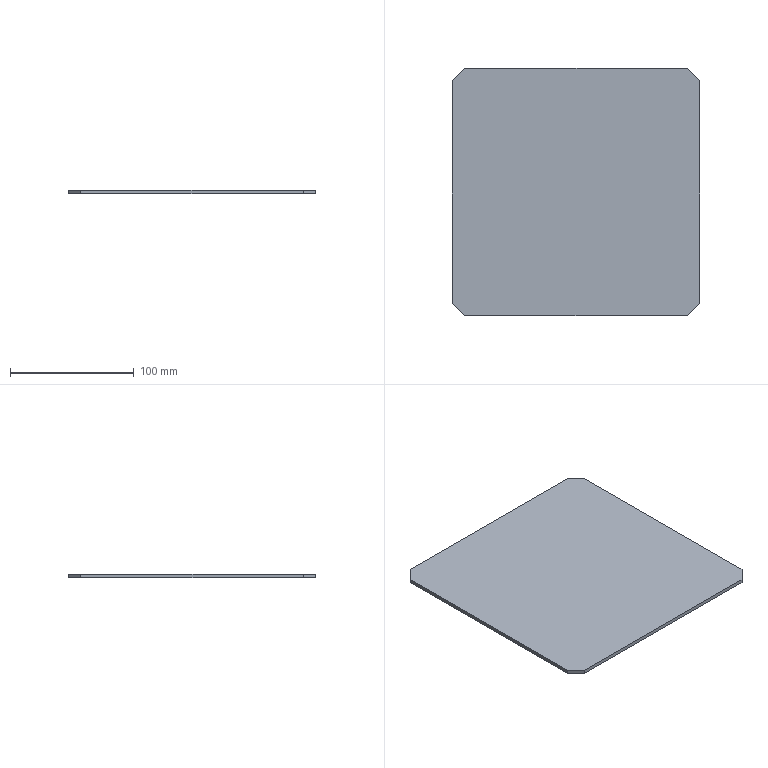Part | SolidWorks | features Chamfer 1, Extrusion 1 | 1 solid | 10 faces | box 200 x 200 x 3 mm | volume 119400 mm3 | plane 10
STEP:
#1=CARTESIAN_POINT('',(100.,-90.,3.));
#2=VERTEX_POINT('',#1);
#3=CARTESIAN_POINT('',(100.,90.,3.));
#4=VERTEX_POINT('',#3);
#5=CARTESIAN_POINT('',(100.,100.,3.));
#6=DIRECTION('',(0.,1.,0.));
#7=VECTOR('',#6,1000.);
#8=LINE('',#5,#7);
#9=EDGE_CURVE('',#2,#4,#8,.T.);
#10=ORIENTED_EDGE('',*,*,#9,.F.);
#11=CARTESIAN_POINT('',(100.,-90.,0.));
#12=VERTEX_POINT('',#11);
#13=CARTESIAN_POINT('',(100.,-90.,3.));
#14=DIRECTION('',(0.,0.,-1.));
#15=VECTOR('',#14,1000.);
#16=LINE('',#13,#15);
#17=EDGE_CURVE('',#2,#12,#16,.T.);
#18=ORIENTED_EDGE('',*,*,#17,.T.);
#19=CARTESIAN_POINT('',(100.,90.,0.));
#20=VERTEX_POINT('',#19);
#21=CARTESIAN_POINT('',(100.,100.,0.));
#22=DIRECTION('',(0.,1.,0.));
#23=VECTOR('',#22,1000.);
#24=LINE('',#21,#23);
#25=EDGE_CURVE('',#12,#20,#24,.T.);
#26=ORIENTED_EDGE('',*,*,#25,.T.);
#27=CARTESIAN_POINT('',(100.,90.,3.));
#28=DIRECTION('',(0.,0.,1.));
#29=VECTOR('',#28,1000.);
#30=LINE('',#27,#29);
#31=EDGE_CURVE('',#20,#4,#30,.T.);
#32=ORIENTED_EDGE('',*,*,#31,.T.);
#33=EDGE_LOOP('',(#10,#18,#26,#32));
#34=FACE_OUTER_BOUND('',#33,.T.);
#35=CARTESIAN_POINT('',(100.,100.,3.));
#36=DIRECTION('',(-1.,0.,0.));
#37=DIRECTION('',(0.,-1.,0.));
#38=AXIS2_PLACEMENT_3D('',#35,#36,#37);
#39=PLANE('',#38);
#40=ADVANCED_FACE('',(#34),#39,.F.);
#41=CARTESIAN_POINT('',(90.,100.,3.));
#42=VERTEX_POINT('',#41);
#43=CARTESIAN_POINT('',(-90.,100.,3.));
#44=VERTEX_POINT('',#43);
#45=CARTESIAN_POINT('',(-100.,100.,3.));
#46=DIRECTION('',(-1.,0.,0.));
#47=VECTOR('',#46,1000.);
#48=LINE('',#45,#47);
#49=EDGE_CURVE('',#42,#44,#48,.T.);
#50=ORIENTED_EDGE('',*,*,#49,.F.);
#51=CARTESIAN_POINT('',(90.,100.,0.));
#52=VERTEX_POINT('',#51);
#53=CARTESIAN_POINT('',(90.,100.,3.));
#54=DIRECTION('',(0.,0.,-1.));
#55=VECTOR('',#54,1000.);
#56=LINE('',#53,#55);
#57=EDGE_CURVE('',#42,#52,#56,.T.);
#58=ORIENTED_EDGE('',*,*,#57,.T.);
#59=CARTESIAN_POINT('',(-90.,100.,0.));
#60=VERTEX_POINT('',#59);
#61=CARTESIAN_POINT('',(-100.,100.,0.));
#62=DIRECTION('',(-1.,0.,0.));
#63=VECTOR('',#62,1000.);
#64=LINE('',#61,#63);
#65=EDGE_CURVE('',#52,#60,#64,.T.);
#66=ORIENTED_EDGE('',*,*,#65,.T.);
#67=CARTESIAN_POINT('',(-90.,100.,3.));
#68=DIRECTION('',(0.,0.,1.));
#69=VECTOR('',#68,1000.);
#70=LINE('',#67,#69);
#71=EDGE_CURVE('',#60,#44,#70,.T.);
#72=ORIENTED_EDGE('',*,*,#71,.T.);
#73=EDGE_LOOP('',(#50,#58,#66,#72));
#74=FACE_OUTER_BOUND('',#73,.T.);
#75=CARTESIAN_POINT('',(-100.,100.,3.));
#76=DIRECTION('',(0.,-1.,0.));
#77=DIRECTION('',(0.,0.,-1.));
#78=AXIS2_PLACEMENT_3D('',#75,#76,#77);
#79=PLANE('',#78);
#80=ADVANCED_FACE('',(#74),#79,.F.);
#81=CARTESIAN_POINT('',(-100.,90.,0.));
#82=VERTEX_POINT('',#81);
#83=CARTESIAN_POINT('',(-100.,-90.,0.));
#84=VERTEX_POINT('',#83);
#85=CARTESIAN_POINT('',(-100.,100.,0.));
#86=DIRECTION('',(0.,-1.,0.));
#87=VECTOR('',#86,1000.);
#88=LINE('',#85,#87);
#89=EDGE_CURVE('',#82,#84,#88,.T.);
#90=ORIENTED_EDGE('',*,*,#89,.T.);
#91=CARTESIAN_POINT('',(-100.,-90.,3.));
#92=VERTEX_POINT('',#91);
#93=CARTESIAN_POINT('',(-100.,-90.,3.));
#94=DIRECTION('',(0.,0.,1.));
#95=VECTOR('',#94,1000.);
#96=LINE('',#93,#95);
#97=EDGE_CURVE('',#84,#92,#96,.T.);
#98=ORIENTED_EDGE('',*,*,#97,.T.);
#99=CARTESIAN_POINT('',(-100.,90.,3.));
#100=VERTEX_POINT('',#99);
#101=CARTESIAN_POINT('',(-100.,100.,3.));
#102=DIRECTION('',(0.,-1.,0.));
#103=VECTOR('',#102,1000.);
#104=LINE('',#101,#103);
#105=EDGE_CURVE('',#100,#92,#104,.T.);
#106=ORIENTED_EDGE('',*,*,#105,.F.);
#107=CARTESIAN_POINT('',(-100.,90.,3.));
#108=DIRECTION('',(0.,0.,-1.));
#109=VECTOR('',#108,1000.);
#110=LINE('',#107,#109);
#111=EDGE_CURVE('',#100,#82,#110,.T.);
#112=ORIENTED_EDGE('',*,*,#111,.T.);
#113=EDGE_LOOP('',(#90,#98,#106,#112));
#114=FACE_OUTER_BOUND('',#113,.T.);
#115=CARTESIAN_POINT('',(-100.,100.,3.));
#116=DIRECTION('',(1.,0.,0.));
#117=DIRECTION('',(0.,1.,0.));
#118=AXIS2_PLACEMENT_3D('',#115,#116,#117);
#119=PLANE('',#118);
#120=ADVANCED_FACE('',(#114),#119,.F.);
#121=CARTESIAN_POINT('',(-90.,-100.,3.));
#122=VERTEX_POINT('',#121);
#123=CARTESIAN_POINT('',(90.,-100.,3.));
#124=VERTEX_POINT('',#123);
#125=CARTESIAN_POINT('',(-100.,-100.,3.));
#126=DIRECTION('',(1.,0.,0.));
#127=VECTOR('',#126,1000.);
#128=LINE('',#125,#127);
#129=EDGE_CURVE('',#122,#124,#128,.T.);
#130=ORIENTED_EDGE('',*,*,#129,.F.);
#131=CARTESIAN_POINT('',(-90.,-100.,0.));
#132=VERTEX_POINT('',#131);
#133=CARTESIAN_POINT('',(-90.,-100.,3.));
#134=DIRECTION('',(0.,0.,-1.));
#135=VECTOR('',#134,1000.);
#136=LINE('',#133,#135);
#137=EDGE_CURVE('',#122,#132,#136,.T.);
#138=ORIENTED_EDGE('',*,*,#137,.T.);
#139=CARTESIAN_POINT('',(90.,-100.,0.));
#140=VERTEX_POINT('',#139);
#141=CARTESIAN_POINT('',(-100.,-100.,0.));
#142=DIRECTION('',(1.,0.,0.));
#143=VECTOR('',#142,1000.);
#144=LINE('',#141,#143);
#145=EDGE_CURVE('',#132,#140,#144,.T.);
#146=ORIENTED_EDGE('',*,*,#145,.T.);
#147=CARTESIAN_POINT('',(90.,-100.,3.));
#148=DIRECTION('',(0.,0.,1.));
#149=VECTOR('',#148,1000.);
#150=LINE('',#147,#149);
#151=EDGE_CURVE('',#140,#124,#150,.T.);
#152=ORIENTED_EDGE('',*,*,#151,.T.);
#153=EDGE_LOOP('',(#130,#138,#146,#152));
#154=FACE_OUTER_BOUND('',#153,.T.);
#155=CARTESIAN_POINT('',(-100.,-100.,3.));
#156=DIRECTION('',(0.,1.,0.));
#157=DIRECTION('',(0.,0.,1.));
#158=AXIS2_PLACEMENT_3D('',#155,#156,#157);
#159=PLANE('',#158);
#160=ADVANCED_FACE('',(#154),#159,.F.);
#161=ORIENTED_EDGE('',*,*,#105,.T.);
#162=CARTESIAN_POINT('',(-95.,-95.,3.));
#163=DIRECTION('',(0.7071,-0.7071,0.));
#164=VECTOR('',#163,1000.);
#165=LINE('',#162,#164);
#166=EDGE_CURVE('',#92,#122,#165,.T.);
#167=ORIENTED_EDGE('',*,*,#166,.T.);
#168=ORIENTED_EDGE('',*,*,#129,.T.);
#169=CARTESIAN_POINT('',(95.,-95.,3.));
#170=DIRECTION('',(0.7071,0.7071,0.));
#171=VECTOR('',#170,1000.);
#172=LINE('',#169,#171);
#173=EDGE_CURVE('',#124,#2,#172,.T.);
#174=ORIENTED_EDGE('',*,*,#173,.T.);
#175=ORIENTED_EDGE('',*,*,#9,.T.);
#176=CARTESIAN_POINT('',(95.,95.,3.));
#177=DIRECTION('',(-0.7071,0.7071,0.));
#178=VECTOR('',#177,1000.);
#179=LINE('',#176,#178);
#180=EDGE_CURVE('',#4,#42,#179,.T.);
#181=ORIENTED_EDGE('',*,*,#180,.T.);
#182=ORIENTED_EDGE('',*,*,#49,.T.);
#183=CARTESIAN_POINT('',(-95.,95.,3.));
#184=DIRECTION('',(-0.7071,-0.7071,0.));
#185=VECTOR('',#184,1000.);
#186=LINE('',#183,#185);
#187=EDGE_CURVE('',#44,#100,#186,.T.);
#188=ORIENTED_EDGE('',*,*,#187,.T.);
#189=EDGE_LOOP('',(#161,#167,#168,#174,#175,#181,#182,#188));
#190=FACE_OUTER_BOUND('',#189,.T.);
#191=CARTESIAN_POINT('',(0.,0.,3.));
#192=DIRECTION('',(0.,0.,1.));
#193=DIRECTION('',(1.,0.,0.));
#194=AXIS2_PLACEMENT_3D('',#191,#192,#193);
#195=PLANE('',#194);
#196=ADVANCED_FACE('',(#190),#195,.T.);
#197=ORIENTED_EDGE('',*,*,#145,.F.);
#198=CARTESIAN_POINT('',(-90.,-100.,0.));
#199=DIRECTION('',(-0.7071,0.7071,0.));
#200=VECTOR('',#199,1000.);
#201=LINE('',#198,#200);
#202=EDGE_CURVE('',#132,#84,#201,.T.);
#203=ORIENTED_EDGE('',*,*,#202,.T.);
#204=ORIENTED_EDGE('',*,*,#89,.F.);
#205=CARTESIAN_POINT('',(-100.,90.,0.));
#206=DIRECTION('',(0.7071,0.7071,0.));
#207=VECTOR('',#206,1000.);
#208=LINE('',#205,#207);
#209=EDGE_CURVE('',#82,#60,#208,.T.);
#210=ORIENTED_EDGE('',*,*,#209,.T.);
#211=ORIENTED_EDGE('',*,*,#65,.F.);
#212=CARTESIAN_POINT('',(90.,100.,0.));
#213=DIRECTION('',(0.7071,-0.7071,0.));
#214=VECTOR('',#213,1000.);
#215=LINE('',#212,#214);
#216=EDGE_CURVE('',#52,#20,#215,.T.);
#217=ORIENTED_EDGE('',*,*,#216,.T.);
#218=ORIENTED_EDGE('',*,*,#25,.F.);
#219=CARTESIAN_POINT('',(100.,-90.,0.));
#220=DIRECTION('',(-0.7071,-0.7071,0.));
#221=VECTOR('',#220,1000.);
#222=LINE('',#219,#221);
#223=EDGE_CURVE('',#12,#140,#222,.T.);
#224=ORIENTED_EDGE('',*,*,#223,.T.);
#225=EDGE_LOOP('',(#197,#203,#204,#210,#211,#217,#218,#224));
#226=FACE_OUTER_BOUND('',#225,.T.);
#227=CARTESIAN_POINT('',(0.,0.,0.));
#228=DIRECTION('',(0.,0.,1.));
#229=DIRECTION('',(1.,0.,0.));
#230=AXIS2_PLACEMENT_3D('',#227,#228,#229);
#231=PLANE('',#230);
#232=ADVANCED_FACE('',(#226),#231,.F.);
#233=ORIENTED_EDGE('',*,*,#166,.F.);
#234=ORIENTED_EDGE('',*,*,#97,.F.);
#235=ORIENTED_EDGE('',*,*,#202,.F.);
#236=ORIENTED_EDGE('',*,*,#137,.F.);
#237=EDGE_LOOP('',(#233,#234,#235,#236));
#238=FACE_OUTER_BOUND('',#237,.T.);
#239=CARTESIAN_POINT('',(-90.,-100.,3.));
#240=DIRECTION('',(0.7071,0.7071,0.));
#241=DIRECTION('',(0.,0.,-1.));
#242=AXIS2_PLACEMENT_3D('',#239,#240,#241);
#243=PLANE('',#242);
#244=ADVANCED_FACE('',(#238),#243,.F.);
#245=ORIENTED_EDGE('',*,*,#173,.F.);
#246=ORIENTED_EDGE('',*,*,#151,.F.);
#247=ORIENTED_EDGE('',*,*,#223,.F.);
#248=ORIENTED_EDGE('',*,*,#17,.F.);
#249=EDGE_LOOP('',(#245,#246,#247,#248));
#250=FACE_OUTER_BOUND('',#249,.T.);
#251=CARTESIAN_POINT('',(100.,-90.,3.));
#252=DIRECTION('',(-0.7071,0.7071,0.));
#253=DIRECTION('',(0.,0.,-1.));
#254=AXIS2_PLACEMENT_3D('',#251,#252,#253);
#255=PLANE('',#254);
#256=ADVANCED_FACE('',(#250),#255,.F.);
#257=ORIENTED_EDGE('',*,*,#180,.F.);
#258=ORIENTED_EDGE('',*,*,#31,.F.);
#259=ORIENTED_EDGE('',*,*,#216,.F.);
#260=ORIENTED_EDGE('',*,*,#57,.F.);
#261=EDGE_LOOP('',(#257,#258,#259,#260));
#262=FACE_OUTER_BOUND('',#261,.T.);
#263=CARTESIAN_POINT('',(90.,100.,3.));
#264=DIRECTION('',(-0.7071,-0.7071,0.));
#265=DIRECTION('',(0.,0.,-1.));
#266=AXIS2_PLACEMENT_3D('',#263,#264,#265);
#267=PLANE('',#266);
#268=ADVANCED_FACE('',(#262),#267,.F.);
#269=ORIENTED_EDGE('',*,*,#187,.F.);
#270=ORIENTED_EDGE('',*,*,#71,.F.);
#271=ORIENTED_EDGE('',*,*,#209,.F.);
#272=ORIENTED_EDGE('',*,*,#111,.F.);
#273=EDGE_LOOP('',(#269,#270,#271,#272));
#274=FACE_OUTER_BOUND('',#273,.T.);
#275=CARTESIAN_POINT('',(-100.,90.,3.));
#276=DIRECTION('',(0.7071,-0.7071,0.));
#277=DIRECTION('',(0.,0.,-1.));
#278=AXIS2_PLACEMENT_3D('',#275,#276,#277);
#279=PLANE('',#278);
#280=ADVANCED_FACE('',(#274),#279,.F.);
#281=CLOSED_SHELL('',(#40,#80,#120,#160,#196,#232,#244,#256,#268,#280));
#282=MANIFOLD_SOLID_BREP('',#281);
#283=CARTESIAN_POINT('',(0.,0.,0.));
#284=DIRECTION('',(0.,0.,1.));
#285=DIRECTION('',(1.,0.,0.));
#286=AXIS2_PLACEMENT_3D('',#283,#284,#285);
#287=(LENGTH_UNIT()NAMED_UNIT(*)SI_UNIT(.MILLI.,.METRE.));
#288=UNCERTAINTY_MEASURE_WITH_UNIT(LENGTH_MEASURE(0.00001),#287,'','');
#289=(NAMED_UNIT(*)PLANE_ANGLE_UNIT()SI_UNIT($,.RADIAN.));
#290=(NAMED_UNIT(*)SI_UNIT($,.STERADIAN.)SOLID_ANGLE_UNIT());
#291=(GEOMETRIC_REPRESENTATION_CONTEXT(3)GLOBAL_UNCERTAINTY_ASSIGNED_CONTEXT((#288))GLOBAL_UNIT_ASSIGNED_CONTEXT((#287,#289,#290))REPRESENTATION_CONTEXT('',''));
#292=ADVANCED_BREP_SHAPE_REPRESENTATION('',(#282,#286),#291);